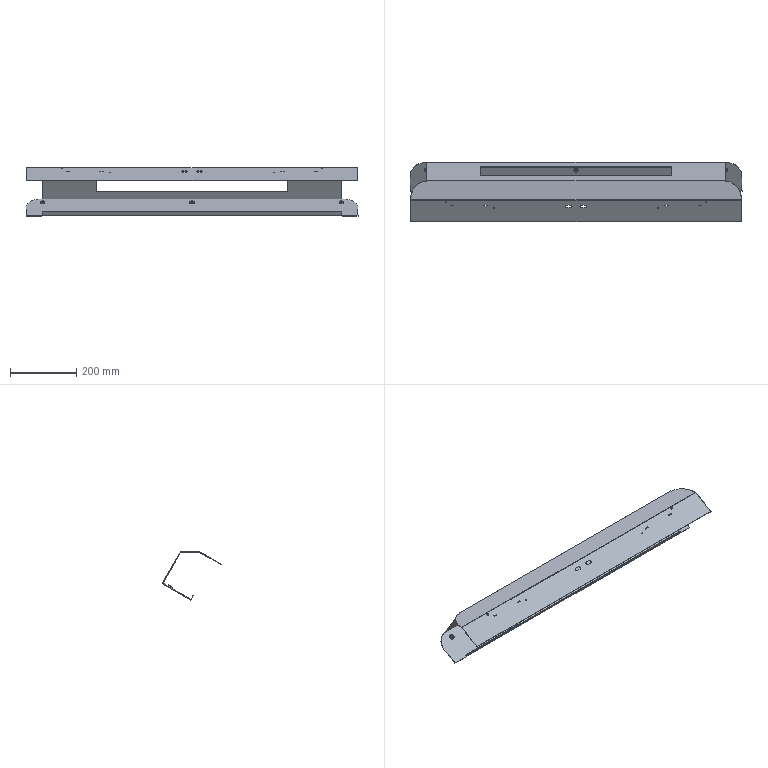Part | STEP file | FHD-021-001-G rack welded part G | 1 solid | 83 faces | box 1000 x 178.631 x 144.83 mm | volume 461158 mm3 | plane 55 | cylinder 24 | spline 4 | commonest cylinder face diameters 0.4 x4 3.4 x4 9 x4 6.8 x3 13 x3 2.5 x2